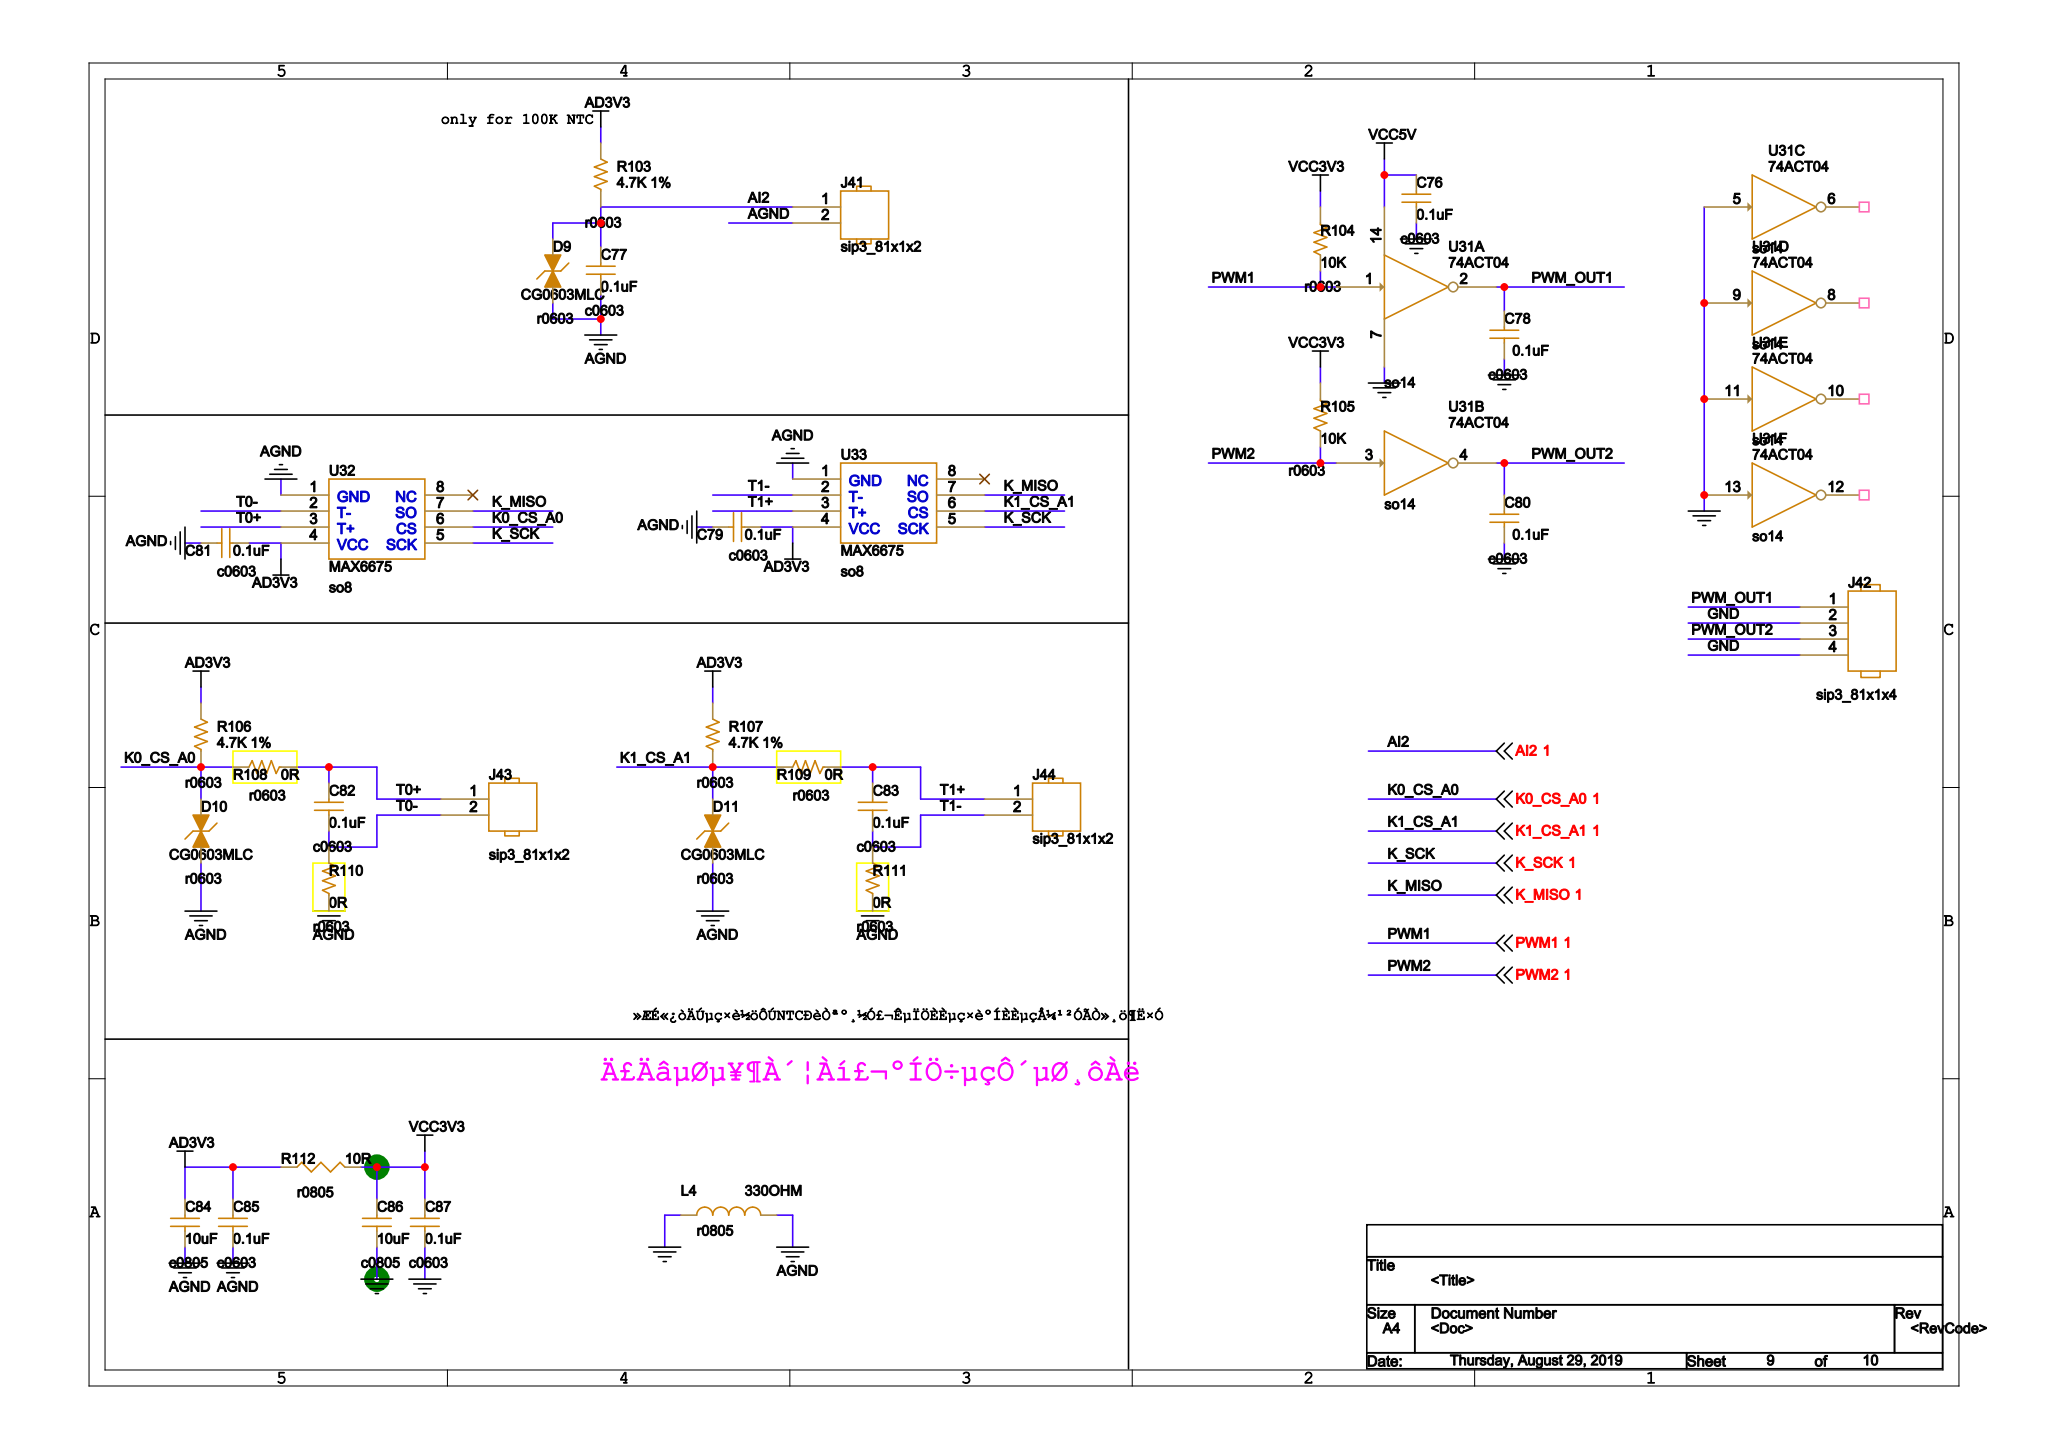Circuit board | Cadence Allegro | 380 parts | 375 nets | one sheet of the schematic
Parts on this sheet (reference | value | footprint):
C76 | 0.1uF | C0603
C77 | 0.1uF | C0603
C78 | 0.1uF | C0603
C79 | 0.1uF | C0603
C80 | 0.1uF | C0603
C81 | 0.1uF | C0603
C82 | 0.1uF | C0603
C83 | 0.1uF | C0603
C84 | 10uF | C0805
C85 | 0.1uF | C0603
C86 | 10uF | C0805
C87 | 0.1uF | C0603
D9 | CG0603MLC | R0603
D10 | CG0603MLC | R0603
D11 | CG0603MLC | R0603
J41 | HEADER 2 | SIP3_81X1X2
J42 | HEADER 4 | SIP3_81X1X4
J43 | HEADER 2 | SIP3_81X1X2
J44 | HEADER 2 | SIP3_81X1X2
L4 | 330OHM | R0805
R103 | 4.7K 1% | R0603
R104 | 10K | R0603
R105 | 10K | R0603
R106 | 4.7K 1% | R0603
R107 | 4.7K 1% | R0603
R108 | 0R | R0603
R109 | 0R | R0603
R110 | 0R | R0603
R111 | 0R | R0603
R112 | 10R | R0805
U32 | MAX6675 | SO8
U33 | MAX6675 | SO8
Nets of these parts (net: part-pin ...):
GND: C76-2 C78-2 C80-2 C86-2 C87-2 J42-2 J42-4 L4-1
VCC3V3: C86-1 C87-1 R104-1 R105-1 R112-2
VCC5V: C76-1
AI2: C77-1 D9-1 J41-1 R103-1
AD3V3: C79-1 C81-1 C84-1 C85-1 R103-2 R106-2 R107-2 R112-1 U32-4 U33-4
K0_CS_A0: D10-1 R106-1 R108-2 U32-6
K1_CS_A1: D11-1 R107-1 R109-2 U33-6
PWM_OUT1: C78-1 J42-1
AGND: C77-2 C79-2 C81-2 C84-2 C85-2 D9-2 D10-2 D11-2 J41-2 L4-2 R110-1 R111-1 U32-1 U33-1
PWM_OUT2: C80-1 J42-3
T0+: C82-1 J43-1 R108-1 U32-3
T0-: C82-2 J43-2 R110-2 U32-2
T1+: C83-1 J44-1 R109-1 U33-3
T1-: C83-2 J44-2 R111-2 U33-2
PWM1: R104-2
PWM2: R105-2
K_MISO: U32-7 U33-7
K_SCK: U32-5 U33-5